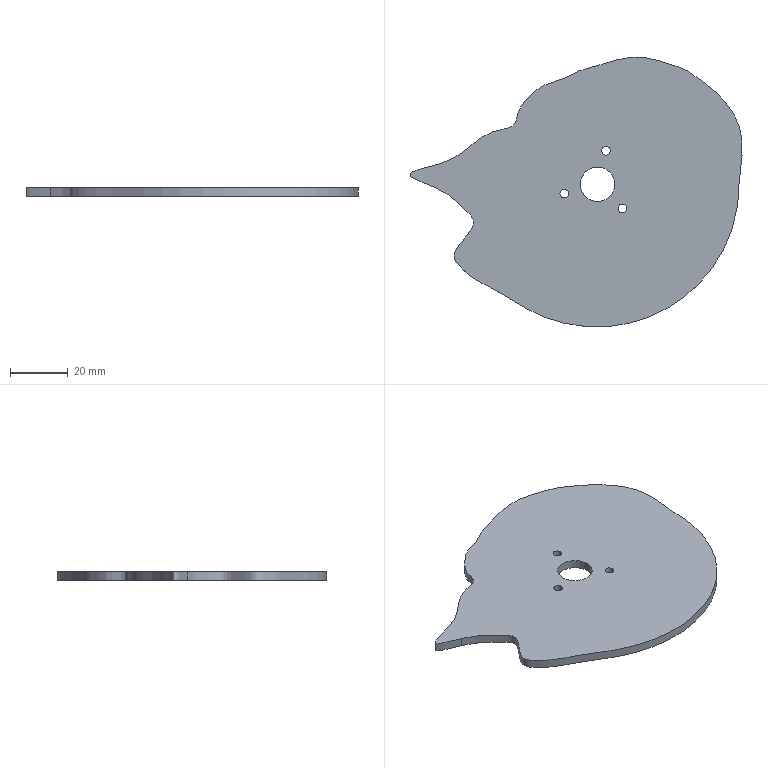Part | SolidWorks | features ICE 2, CurveInFile 1, Extrusion 1 | 1 solid | 12 faces | box 115.273 x 93.626 x 3 mm | volume 21562 mm3 | cylinder 8 | spline 2 | plane 2 | commonest cylinder face diameters 3 x6 12 x2